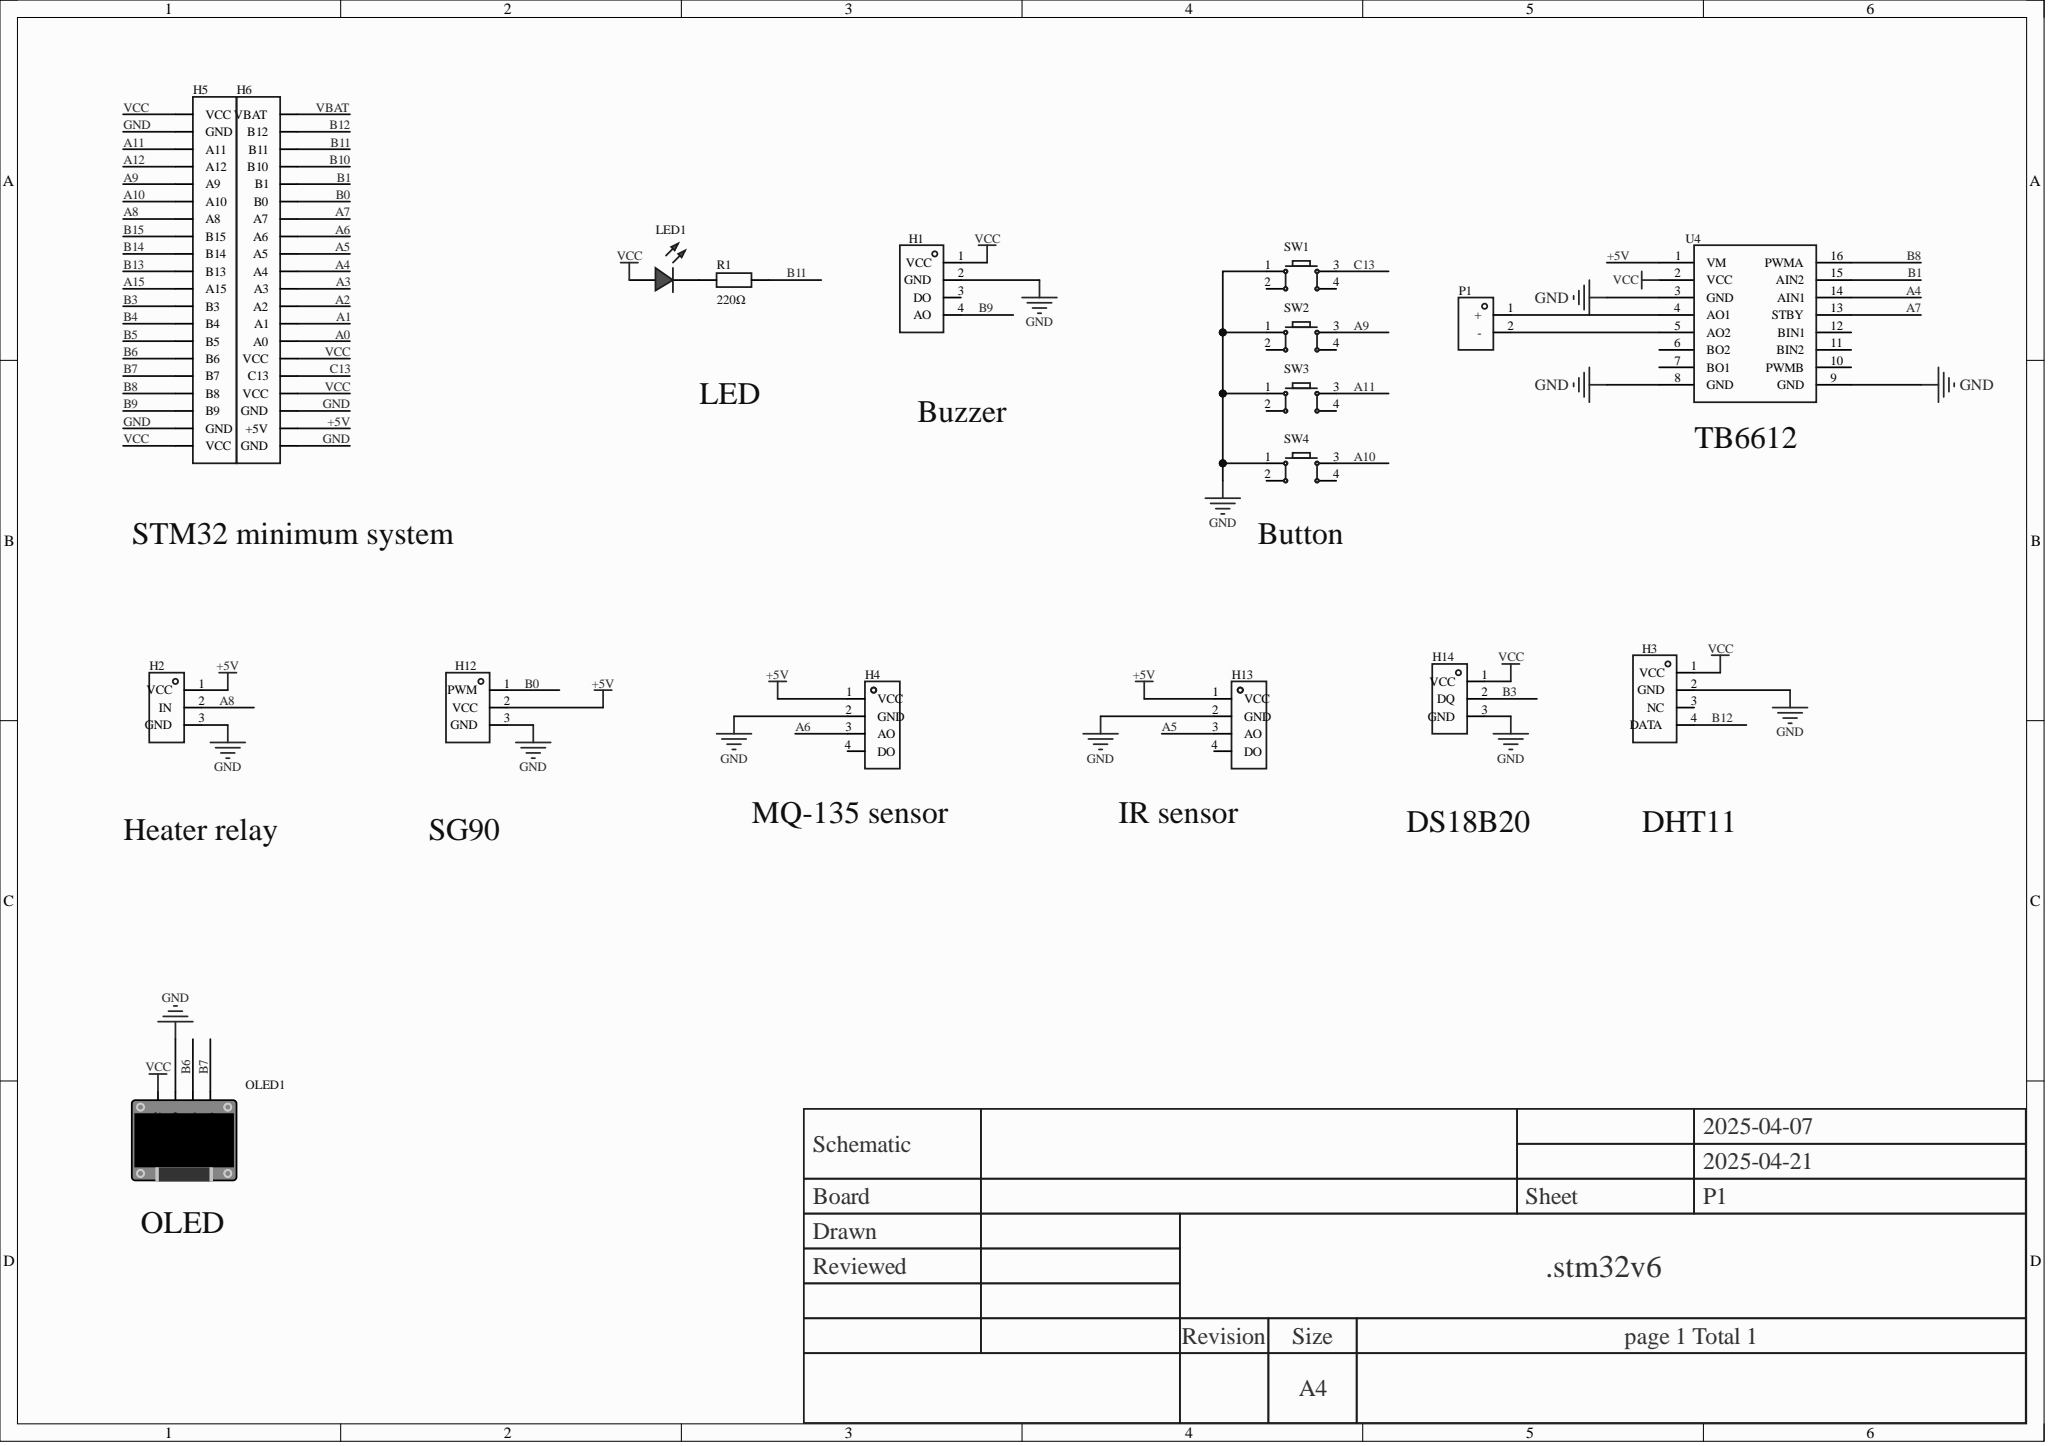Circuit board | Altium Designer | 18 parts | 24 nets
Bill of materials:
Comment,Description,Designator,Footprint,LibRef,Quantity
"","","H1, H3, H4, H13","HDR-TH_4P-P2.54-V-F","HDR-F_2.54_1x4P","4"
"","","H2, H12, H14","HDR-TH_3P-P2.54-V-F","HDR-F_2.54_1x3P","3"
"","","H5, H6","HDR-TH_20P-P2.54-V-F","HDR-F_2.54_1x20P","2"
"","","LED1","LED_TH-3mm","LED_TH-R_3mm","1"
"","","OLED1","0.96OLED_4P","0.96OLED模块_4P","1"
"KF301-2P terminal block","","P1","CONN-TH_XY301V-A-5.0-2P","KF301-2P接线端子","1"
"220Ω","","R1","Res_1/8W","Res_AXIAL-1/8W","1"
"","","SW1, SW2, SW3, SW4","SW-TH_4P-L6.0-W6.0-P4.50-LS6.5","Key_TH_6x6x6","4"
"","","U4","tb6612","tb6612","1"
Netlist (Protel format):
[
H1
HDR-TH_4P-P2.54-V-F




]
[
H2
HDR-TH_3P-P2.54-V-F




]
[
H3
HDR-TH_4P-P2.54-V-F




]
[
H4
HDR-TH_4P-P2.54-V-F




]
[
H5
HDR-TH_20P-P2.54-V-F




]
[
H6
HDR-TH_20P-P2.54-V-F




]
[
H12
HDR-TH_3P-P2.54-V-F




]
[
H13
HDR-TH_4P-P2.54-V-F




]
[
H14
HDR-TH_3P-P2.54-V-F




]
[
LED1
LED_TH-3mm




]
[
OLED1
0.96OLED_4P




]
[
P1
CONN-TH_XY301V-A-5.0-2P
KF301-2P terminal block



]
[
R1
Res_1/8W
220Ω



]
[
SW1
SW-TH_4P-L6.0-W6.0-P4.50-LS6.5




]
[
SW2
SW-TH_4P-L6.0-W6.0-P4.50-LS6.5




]
[
SW3
SW-TH_4P-L6.0-W6.0-P4.50-LS6.5




]
[
SW4
SW-TH_4P-L6.0-W6.0-P4.50-LS6.5




]
[
U4
tb6612




]
(
VCC
H1-1
H3-1
H5-1
H5-20
H6-15
H6-17
H14-1
LED1-1
OLED1-1
U4-2
)
(
NetP1_2
P1-2
U4-5
)
(
NetP1_1
P1-1
U4-4
)
(
NetLED1_2
LED1-2
R1-1
)
(
GND
H1-2
H2-3
H3-2
H4-2
H5-2
H5-19
H6-18
H6-20
H12-3
H13-2
H14-3
OLED1-2
SW1-1
SW2-1
SW3-1
SW4-1
U4-3
U4-8
U4-9
)
(
C13
H6-16
SW1-3
)
(
B12
H3-4
H6-2
)
(
B11
H6-3
R1-2
)
(
B9
H1-4
H5-18
)
(
B8
H5-17
U4-16
)
(
B7
H5-16
OLED1-4
)
(
B6
H5-15
OLED1-3
)
(
B3
H5-12
H14-2
)
(
B1
H6-5
U4-15
)
(
B0
H6-6
H12-1
)
(
A11
H5-3
SW3-3
)
(
A10
H5-6
SW4-3
)
(
A9
H5-5
SW2-3
)
(
A8
H2-2
H5-7
)
(
A7
H6-7
U4-13
)
(
A6
H4-3
H6-8
)
(
A5
H6-9
H13-3
)
(
A4
H6-10
U4-14
)
(
+5V
H2-1
H4-1
H6-19
H12-2
H13-1
U4-1
)